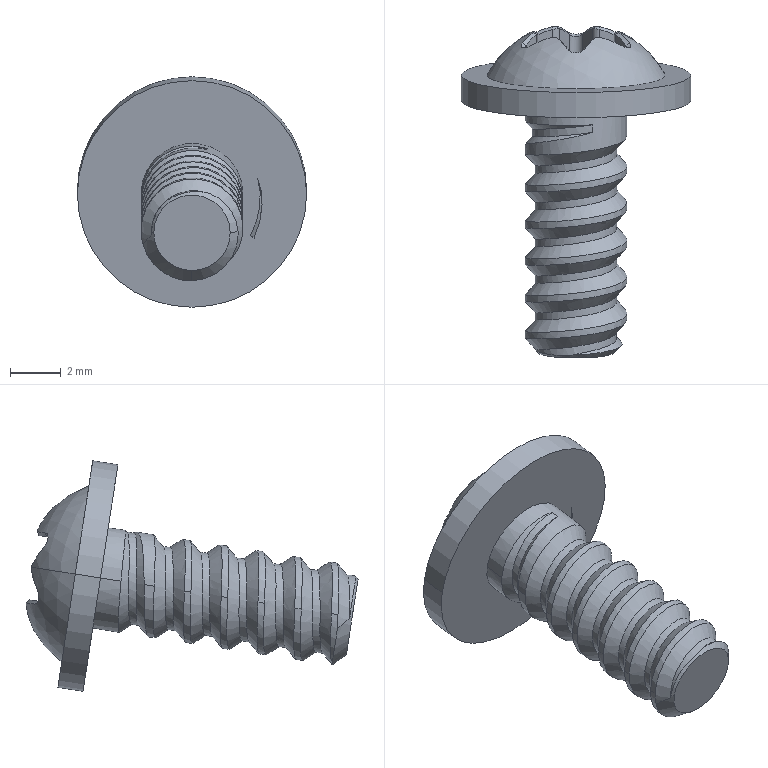Part | SolidWorks | features BaseBody 1 | 1 solid | 90 faces | box 9 x 13.034 x 9.047 mm | volume 194.188 mm3 | cylinder 27 | spline 25 | cone 17 | plane 16 | sphere 5 | commonest cylinder face diameters 4 x13 0.6 x12 9 x2